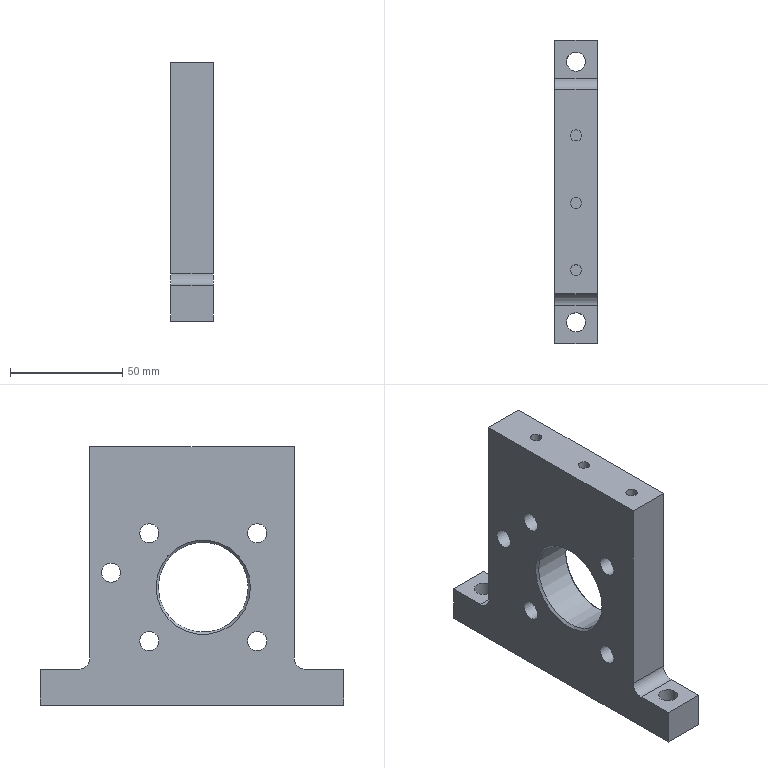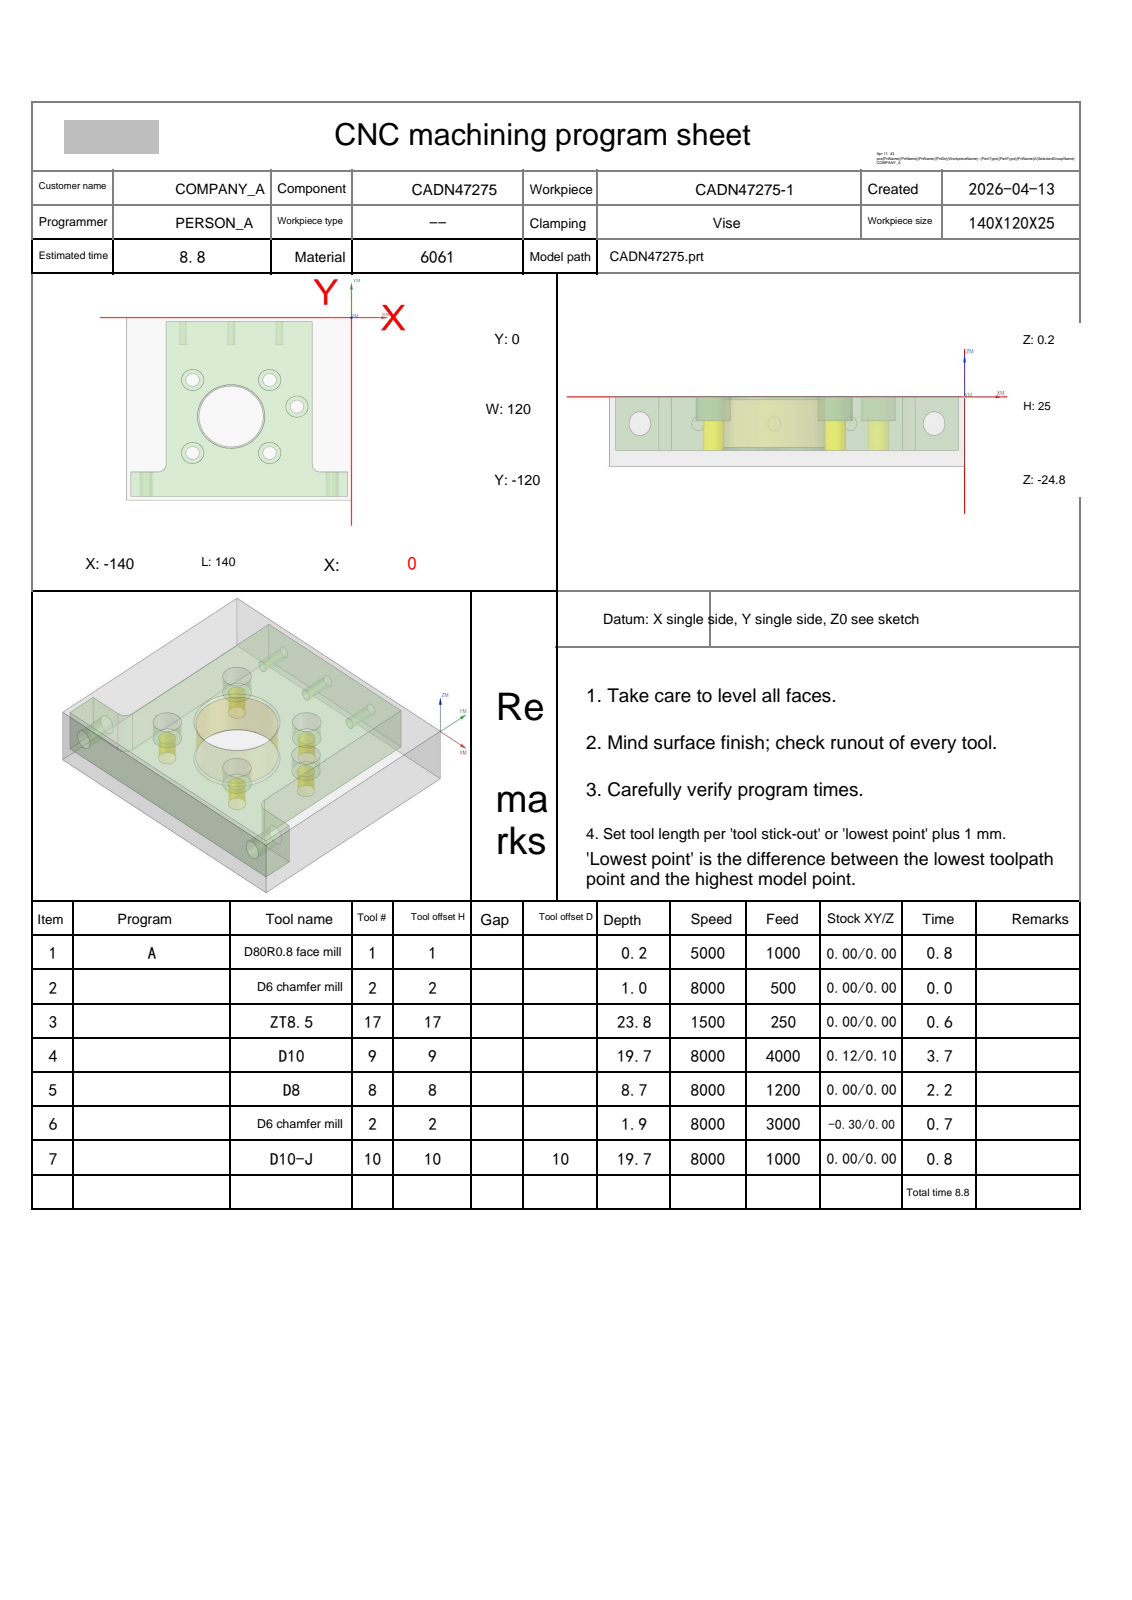NC program | NX | posted by the shop | part box 19 x 135 x 115 mm
Lines 73 to 878 of 2456:
N4 T09 M06
(D10  D=10. R=0. H=09 ce=0.12 di=0.10)
G00 G90 G54 X-117.765 Y10.948 M03 S8000
G43 H09 Z20.
M08
Z-17.5
G01 X-117.749 Y10.849 Z-18.125 F4000.
X-117.733 Y10.75 Z-18.372
X-117.717 Y10.651 Z-18.554
X-117.701 Y10.553 Z-18.7
X-117.686 Y10.454 Z-18.823
X-117.67 Y10.355 Z-18.928
X-117.654 Y10.256 Z-19.02
X-117.638 Y10.158 Z-19.1
X-117.622 Y10.059 Z-19.17
X-117.606 Y9.96 Z-19.232
X-117.591 Y9.861 Z-19.286
X-117.575 Y9.763 Z-19.333
X-117.559 Y9.664 Z-19.374
X-117.543 Y9.565 Z-19.408
X-117.527 Y9.466 Z-19.436
X-117.511 Y9.368 Z-19.46
X-117.496 Y9.269 Z-19.477
X-117.48 Y9.17 Z-19.49
X-117.464 Y9.072 Z-19.497
X-117.448 Y8.973 Z-19.5
X-117.115 Y6.898
G03 X-116.786 Y6.503 I.503 J.083
X-112.933 Y5.928 I3.896 J12.905
X-103.721 Y5.791 I9.212 J309.636
X-101.259 Y5.8 I0.0 J309.773
G01 X-1.649 Y5.779
G02 X4.276 Y1.747 I-.206 J-6.674
X5.587 Y-3.961 I-14.753 J-6.393
X5.818 Y-12.935 I-174.896 J-8.974
X5.799 Y-15.507 I-175.126 J0.0
G01 X5.781 Y-118.297
G02 X1.748 Y-124.273 I-6.683 J.161
X-4.16 Y-125.602 I-6.488 J15.041
X-12.594 Y-125.81 I-8.434 J170.831
X-14.656 Y-125.798 I0.0 J171.039
G01 X-138.297 Y-125.781
G02 X-144.238 Y-121.823 I.146 J6.657
X-145.585 Y-116.06 I14.526 J6.436
X-145.813 Y-107.504 I160.495 J8.556
X-145.798 Y-105.284 I160.723 J0.0
G01 X-145.781 Y-1.693
G02 X-141.823 Y4.238 I6.655 J-.155
X-136.06 Y5.585 I6.436 J-14.523
X-127.504 Y5.813 I8.556 J-160.448
X-125.284 Y5.798 I0.0 J-160.676
X-123.011 Y5.822 I2.274 J-109.436
X-118.506 Y5.729 I0.0 J-109.459
G03 X-106.031 Y5.096 I12.475 J122.585
X-104.399 Y5.107 I0.0 J123.218
G01 X-3.411 Y5.075
G02 X3.002 Y.933 I-.447 J-7.728
X4.757 Y-5.231 I-14.161 J-7.365
X5.1 Y-13.496 I-99.345 J-8.265
X5.092 Y-14.811 I-99.688 J0.0
G01 X5.074 Y-116.58
G02 X.94 Y-122.995 I-7.729 J.44
X-5.348 Y-124.769 I-7.415 J14.255
X-14.012 Y-125.108 I-8.663 J110.618
X-15.769 Y-125.094 I0.0 J110.957
G01 X-136.58 Y-125.075
G02 X-142.999 Y-120.933 I.442 J7.732
X-144.763 Y-114.711 I14.206 J7.389
X-145.108 Y-106.007 I109.485 J8.704
X-145.094 Y-104.22 I109.83 J0.0
G01 X-145.075 Y-3.421
G02 X-140.934 Y2.999 I7.732 J-.442
X-134.711 Y4.763 I7.389 J-14.206
X-126.007 Y5.108 I8.704 J-109.476
X-124.22 Y5.094 I0.0 J-109.822
X-123.6 Y5.096 I.621 J-97.505
X-114.73 Y4.692 I0.0 J-97.507
G03 X-101.233 Y4.378 I13.497 J290.058
X-97.619 Y4.4 I0.0 J290.372
G01 X-5.229 Y4.376
G02 X2.335 Y-.655 I-.393 J-8.793
X4.053 Y-7.188 I-16.636 J-7.866
X4.409 Y-16.533 I-122.28 J-9.345
X4.394 Y-18.449 I-122.636 J0.0
G01 X4.382 Y-114.618
G02 X-.61 Y-122.312 I-8.787 J.235
X-7.415 Y-124.077 I-7.997 J16.841
X-16.317 Y-124.402 I-8.902 J121.564
X-17.836 Y-124.393 I0.0 J121.89
G01 X-134.726 Y-124.377
G02 X-142.28 Y-119.452 I.335 J8.769
X-144.063 Y-112.726 I16.488 J7.97
X-144.403 Y-103.746 I118.292 J8.98
X-144.393 Y-102.165 I118.632 J0.0
G01 X-144.378 Y-5.296
G02 X-139.442 Y2.284 I8.772 J-.316
X-132.847 Y4.049 I7.909 J-16.35
X-124.174 Y4.389 I8.673 J-110.21
X-115.157 Y4.021 I0.0 J-110.55
G03 X-100.288 Y3.681 I14.869 J324.895
X-96.709 Y3.701 I0.0 J325.236
G01 X-7.049 Y3.681
G02 X1.652 Y-2.054 I-.105 J-9.628
X3.357 Y-8.949 I-18.697 J-8.279
X3.703 Y-18.312 I-126.459 J-9.363
X3.692 Y-19.93 I-126.806 J0.0
G01 X3.673 Y-113.09
G02 X2.629 Y-117.342 I-10.374 J.293
G01 X2.446 Y-118.825
X1.934 Y-120.06
X1.12 Y-121.12
X.06 Y-121.934
X-1.175 Y-122.446
G02 X-7.426 Y-123.31 I-30.17 J195.191
X-16.688 Y-123.691 I-9.262 J112.323
X-17.845 Y-123.685 I0.0 J112.704
G01 X-133.055 Y-123.675
G02 X-137.306 Y-122.637 I.246 J10.232
G01 X-138.825 Y-122.446
X-140.06 Y-121.934
X-141.12 Y-121.12
X-141.934 Y-120.06
X-142.446 Y-118.825
G02 X-143.325 Y-112.412 I170.804 J26.702
X-143.69 Y-103.297 I113.665 J9.114
X-143.685 Y-102.201 I114.03 J0.0
G01 X-143.675 Y-6.942
G02 X-138.045 Y1.605 I9.591 J-.19
X-130.95 Y3.366 I8.398 J-18.657
X-123.494 Y3.643 I7.456 J-100.085
X-116.15 Y3.374 I0.0 J-100.362
G03 X-100.164 Y2.992 I15.985 J333.927
X-97.476 Y3.003 I0.0 J334.31
G01 X-8.589 Y2.979
X-8.52
G02 X.904 Y-3.204 I0.0 J-10.273
X2.638 Y-10.315 I-19.87 J-8.614
X3.005 Y-20.222 I-133.631 J-9.907
X2.992 Y-22.066 I-133.997 J0.0
G01 X2.975 Y-111.446
G02 X2.62 Y-114.231 I-16.771 J.721
G01 Y-117.451
X2.6 Y-101.248
G02 X2.418 Y-92.233 I223.082 J9.015
X2.438 Y-89.199 I223.264 J0.0
G01 X2.412 Y-18.929
G03 X2.416 Y-18.177 I-74.932 J.752
X1.871 Y-9.151 I-74.936 J0.0
X-.404 Y-2.515 I-16.313 J-1.884
X-7.619 Y1.981 I-8.589 J-5.744
X-14.302 Y2.433 I-6.683 J-49.236
X-15.228 Y2.424 I0.0 J-49.687
G01 X-23.232 Y2.453
X-24.498 Y2.62
X-111.45 Y2.637
G03 X-122.827 Y3.064 I-32.033 J-701.248
X-124.452 Y3.087 I-1.624 J-58.302
X-132.808 Y2.485 I0.0 J-58.324
X-139. Y.03 I1.969 J-14.001
X-142.642 Y-6.263 I6.083 J-7.72
X-143.124 Y-12.812 I44.253 J-6.549
X-143.117 Y-13.589 I44.735 J0.0
G01 X-143.122 Y-102.549
G03 X-143.124 Y-103.244 I102.156 J-.695
X-142.62 Y-113.38 I102.159 J0.0
X-142.622 Y-114.241 I206.235 J-.861
X-142.593 Y-117.707 I206.237 J0.0
G02 X-142.644 Y-109.06 I731.512 J8.646
X-142.602 Y-101.255 I731.563 J0.0
G03 X-142.42 Y-91.963 I-236.462 J9.292
X-142.439 Y-88.959 I-236.644 J0.0
G01 X-142.411 Y-13.799
G02 X-142.417 Y-13.147 I36.869 J.652
X-141.884 Y-6.9 I36.875 J0.0
X-135.596 Y.566 I10.06 J-2.091
X-128.166 Y2.152 I8.497 J-21.614
X-122.442 Y2.315 I5.724 J-100.129
X-117.463 Y2.192 I0.0 J-100.293
G01 X-116.825 Y2.446
X-115.5 Y2.62
X-110.6
X-115.5
X-116.825 Y2.446
G02 X-119.457 Y1.884 I-2.632 J5.889
G01 X-119.521
G03 X-127.461 Y1.602 I8.321 J-345.796
X-134.633 Y.146 I.995 J-23.303
X-141.052 Y-7.4 I3.89 J-9.811
X-141.812 Y-14.379 I31.689 J-6.979
G01 X-141.811 Y-14.416
G03 X-141.878 Y-23.452 I611.6 J-9.036
G01 Y-23.935
X-141.903 Y-96.2
X-141.986 Y-99.065
X-142.446 Y-100.175
X-142.62 Y-101.498
X-142.446 Y-100.175
G03 X-141.369 Y-95.763 I-9.61 J4.682
X-141.157 Y-86.224 I-214.123 J9.539
X-141.179 Y-83.149 I-214.336 J0.0
G01 X-141.153 Y-17.299
G02 X-141.158 Y-16.586 I47.599 J.713
X-140.605 Y-9.348 I47.605 J0.0
X-133.325 Y-.537 I10.988 J-1.667
X-125.581 Y.915 I8.624 J-24.603
G03 X-119.221 Y1.285 I-3.802 J120.446
X-118.746 Y1.408 I-.724 J3.774
G02 X-117.413 Y2.202 I2.466 J-2.623
G03 X-118.861 Y1.327 I1.415 J-3.975
G02 X-122.098 Y.648 I-3.695 J9.56
G03 X-129.166 Y-.107 I5.054 J-80.754
X-135.663 Y-2.748 I2.192 J-14.706
X-139.753 Y-9.419 I7.358 J-9.102
X-140.551 Y-17. I35.609 J-7.581
G01 Y-17.062
G03 X-140.621 Y-26.574 I650.029 J-9.512
X-140.619 Y-28.262 I650.098 J0.0
G01 X-140.64 Y-89.905
G02 X-140.634 Y-90.696 I-51.361 J-.791
X-141.032 Y-97.077 I-51.367 J0.0
X-141.289 Y-98.099 I-9.752 J1.908
G01 X-141.934 Y-98.94
G03 X-140.422 Y-95.635 I-4.312 J3.971
X-139.944 Y-88.558 I-52.134 J7.077
X-139.949 Y-87.862 I-52.612 J0.0
G01 X-139.919 Y-80.069
X-139.896 Y-20.299
G02 X-139.901 Y-19.504 I57.612 J.795
X-139.372 Y-11.713 I57.618 J0.0
X-136.544 Y-5.179 I12.864 J-1.688
X-129.85 Y-1.255 I9.751 J-8.962
X-122.83 Y-.138 I11.027 J-46.668
G03 X-119.582 Y.565 I-.917 J12.106
G01 X-119.12 Y1.12
X-118.787 Y1.376
G03 X-119.568 Y.549 I1.666 J-2.353
G02 X-122.371 Y-.46 I-3.785 J6.115
G03 X-128.451 Y-1.565 I21.205 J-133.959
X-134.951 Y-4.83 I2.834 J-13.749
X-138.541 Y-11.604 I9.17 J-9.198
X-139.296 Y-19.534 I41.283 J-7.931
G01 Y-19.605
G03 X-139.362 Y-28.974 I663.981 J-9.369
X-139.359 Y-31.085 I664.047 J0.0
G01 X-139.387 Y-87.235
G02 X-139.382 Y-87.963 I-53.015 J-.728
X-139.882 Y-95.231 I-53.02 J0.0
X-140.614 Y-97.486 I-5.927 J.677
G03 X-141.206 Y-97.991 I3.392 J-4.573
G02 X-140.405 Y-97.289 I14.74 J-15.998
G03 X-139.267 Y-94.257 I-5.969 J3.972
X-138.698 Y-86.622 I-50.989 J7.635
X-138.701 Y-86.132 I-51.558 J0.0
G01 X-138.659 Y-76.639
X-138.63 Y-22.199
G02 X-138.634 Y-21.504 I56.935 J.695
X-138.045 Y-13.338 I56.94 J0.0
X-135.069 Y-6.568 I13.543 J-1.916
X-128.639 Y-2.62 I10.123 J-9.278
X-122.69 Y-1.216 I22.71 J-82.942
G03 X-120.094 Y-.232 I-1.362 J7.512
G02 X-119.508 Y.615 I6.338 J-3.753
G03 X-120.062 Y-.228 I2.013 J-1.925
G02 X-122.36 Y-1.48 I-3.707 J4.07
X-127.602 Y-2.946 I-170.119 J597.953
G03 X-133.909 Y-6.609 I3.794 J-13.795
X-137.334 Y-13.709 I10.531 J-9.457
X-138.054 Y-22.224 I49.956 J-8.516
X-138.053 Y-22.627 I50.677 J0.0
G01 X-138.098 Y-33.197
X-138.123 Y-84.303
G02 X-138.118 Y-85.132 I-66.162 J-.829
X-138.631 Y-93.357 I-66.168 J0.0
X-139.784 Y-96.887 I-9.08 J1.014
G01 X-140.615 Y-97.492
G02 X-139.688 Y-96.85 I7.556 J-9.916
G03 X-138.317 Y-94.06 I-4.58 J3.982
X-137.523 Y-87.184 I-32.779 J7.27
X-137.398 Y-77.029 I-413.126 J10.155
X-137.399 Y-76.078 I-413.251 J0.0
G01 X-137.371 Y-24.499
G02 X-137.375 Y-23.813 I63.68 J.686
X-136.81 Y-15.354 I63.684 J0.0
X-133.978 Y-8.337 I14.855 J-1.916
X-127.726 Y-3.994 I10.984 J-9.139
X-122.562 Y-2.227 I219.311 J-632.563
G03 X-120.383 Y-.991 I-1.956 J5.989
G01 X-120.02 Y-.147
G02 X-120.656 Y-1.36 I-3.161 J.885
X-123.65 Y-3.049 I-5.86 J6.888
G03 X-129.001 Y-5.287 I15.603 J-44.831
X-135.744 Y-14.038 I6.275 J-11.808
X-136.739 Y-22.431 I36.853 J-8.623
X-136.841 Y-33.358 I586.61 J-10.927
X-136.838 Y-35.03 I586.712 J0.0
G01 X-136.863 Y-82.133
G02 X-136.859 Y-82.953 I-74.133 J-.82
X-137.394 Y-91.848 I-74.138 J0.0
X-138.784 Y-96.179 I-11.097 J1.171
X-139.284 Y-96.744 I-2.233 J1.473
G01 X-139.93 Y-97.012
G03 X-137.96 Y-95.261 I-.857 J2.948
X-136.595 Y-90.037 I-13.933 J6.431
X-136.142 Y-80.198 I-106.661 J9.839
X-136.15 Y-78.861 I-107.114 J0.0
G01 X-136.111 Y-26.609
G02 X-136.115 Y-25.885 I68.297 J.723
X-135.55 Y-17.114 I68.301 J0.0
X-132.739 Y-9.856 I15.927 J-1.995
X-126.916 Y-5.314 I12.166 J-9.595
G03 X-122.261 Y-3.117 I-40.267 J91.322
X-120.55 Y-1.754 I-2.449 J4.831
G02 X-120.365 Y-.981 I5.741 J-.964
G03 X-120.529 Y-1.76 I2.865 J-1.011
G02 X-122.418 Y-3.567 I-4.172 J2.47
X-127.095 Y-6.075 I-71.012 J126.807
G03 X-134.571 Y-16.003 I6.858 J-12.944
X-135.495 Y-24.829 I42.548 J-8.914
X-135.581 Y-35.581 I671.696 J-10.752
X-135.579 Y-37.358 I671.782 J0.0
G01 X-135.605 Y-80.312
G02 X-135.601 Y-81.068 I-80.89 J-.756
X-136.158 Y-90.54 I-80.893 J0.0
X-137.665 Y-95.46 I-13.433 J1.423
X-138.61 Y-96.515 I-2.353 J1.157
G03 X-139.278 Y-96.742 I1.005 J-4.058
G02 X-138.371 Y-96.435 I5.249 J-14.004
G03 X-136.613 Y-94.133 I-2.8 J3.961
X-135.291 Y-88.226 I-18.857 J7.321
X-134.882 Y-77.993 I-127.868 J10.233
X-134.889 Y-76.694 I-128.276 J0.0
G01 X-134.853 Y-28.699
G02 X-134.858 Y-27.848 I71.97 J.852
X-134.267 Y-18.645 I71.975 J0.0
X-131.423 Y-11.172 I16.89 J-2.151
X-125.809 Y-6.364 I14.236 J-10.94
G03 X-121.657 Y-3.718 I-15.645 J29.138
X-120.62 Y-2.498 I-1.855 J2.628
G01 X-120.51 Y-1.666
G02 X-120.868 Y-3.1 I-3.148 J.023
X-123.427 Y-5.434 I-7.188 J5.311
G03 X-128.253 Y-8.845 I25.166 J-40.716
X-133.408 Y-17.974 I10.642 J-12.03
X-134.25 Y-27.174 I49.857 J-9.201
G01 Y-27.232
G03 X-134.322 Y-37.062 I675.106 J-9.83
X-134.318 Y-39.201 I675.177 J0.0
G01 X-134.342 Y-78.217
G02 X-134.338 Y-79.102 I-91.498 J-.885
X-134.901 Y-89.242 I-91.502 J0.0
X-136.475 Y-94.724 I-16.019 J1.63
X-137.96 Y-96.423 I-3.994 J1.994
G01 X-138.608 Y-96.526
G03 X-136.597 Y-95.433 I-.071 J2.526
X-134.637 Y-90.879 I-8.843 J6.505
X-133.725 Y-81.624 I-49.778 J9.582
X-133.616 Y-69.483 I-680.04 J12.141
X-133.619 Y-67.679 I-680.148 J0.0
G01 X-133.593 Y-30.599
G02 X-133.598 Y-29.747 I77.428 J.852
X-133.024 Y-20.333 I77.433 J0.0
X-130.071 Y-12.33 I18.219 J-2.176
X-125.24 Y-7.643 I16.579 J-12.255
G03 X-121.461 Y-4.592 I-15.484 J23.044
X-120.62 Y-3.311 I-2.183 J2.35
G01 Y-2.498
G02 X-120.597 Y-2.878 I-3.103 J-.379
X-120.74 Y-3.813 I-3.126 J0.0
X-122.888 Y-6.38 I-6.976 J3.656
G03 X-127.248 Y-10.112 I49.65 J-62.404
X-132.236 Y-19.88 I12.635 J-12.609
X-133.008 Y-29.46 I59.051 J-9.58
G01 X-133.007 Y-29.778
X-133.058 Y-40.348
X-133.09 Y-77.368
G02 X-133.088 Y-78.015 I-88.984 J-.646
X-133.71 Y-88.516 I-88.986 J0.0
X-135.406 Y-94.303 I-17.215 J1.904
X-137.277 Y-96.356 I-4.353 J2.09
G01 X-137.984 Y-96.444
G03 X-136.757 Y-96.183 I-.026 J3.141
X-134.502 Y-93.4 I-3.352 J5.022
X-132.906 Y-86.959 I-19.948 J8.361
X-132.369 Y-75.752 I-116.747 J11.208
X-132.376 Y-74.515 I-117.284 J0.0
G01 X-132.335 Y-32.559
G02 X-132.341 Y-31.616 I83.331 J.943
X-131.769 Y-21.872 I83.337 J0.0
X-128.527 Y-13.084 I19.623 J-2.248
X-124.543 Y-8.801 I20.693 J-15.254
G03 X-121.247 Y-5.515 I-15.725 J19.071
X-120.62 Y-4.392 I-2.744 J2.268
G01 Y-3.342
G02 X-120.595 Y-3.82 I-4.597 J-.478
X-120.721 Y-4.892 I-4.622 J0.0
X-122.848 Y-7.823 I-8.328 J3.804
G03 X-127.032 Y-12.235 I38.892 J-41.084
X-131.081 Y-21.879 I16.035 J-12.404
X-131.763 Y-31.776 I71.49 J-9.896
X-131.761 Y-32.348 I72.171 J0.0
G01 X-131.798 Y-41.728
X-131.83 Y-75.83
G02 X-131.828 Y-76.434 I-97.356 J-.604
X-132.443 Y-87.358 I-97.358 J0.0
X-134.217 Y-93.738 I-19.736 J2.051
X-136.536 Y-96.328 I-5.282 J2.396
X-137.116 Y-96.391 I-.58 J2.631
X-137.364 Y-96.38 I0.0 J2.694
G03 X-137.071 Y-96.396 I.293 J2.689
X-134.989 Y-95.418 I0.0 J2.705
X-132.623 Y-90.975 I-7.865 J7.04
X-131.342 Y-82.207 I-37.962 J10.022
X-131.078 Y-68.57 I-351.279 J13.637
X-131.099 Y-64.739 I-351.543 J0.0
G01 X-131.067 Y-33.389
G02 X-131.07 Y-32.708 I77.963 J.681
X-130.443 Y-22.846 I77.966 J0.0
X-124.736 Y-10.903 I21.006 J-2.704
G03 X-121.445 Y-7.153 I-36.854 J35.658
X-120.62 Y-5.66 I-4.069 J3.224
G01 Y-4.4
G02 X-120.606 Y-4.926 I-10.368 J-.526
X-120.662 Y-5.997 I-10.381 J0.0
X-122.432 Y-8.994 I-8.28 J2.868
G03 X-126.296 Y-13.854 I50.804 J-44.367
X-129.897 Y-23.705 I19.228 J-12.61
X-130.511 Y-33.897 I84.208 J-10.191
X-130.508 Y-34.6 I84.823 J0.0
G01 X-130.57 Y-74.43
G02 X-130.569 Y-75.016 I-103.991 J-.586
X-131.193 Y-86.394 I-103.993 J0.0
X-133.028 Y-93.232 I-22.037 J2.247
X-135.59 Y-96.24 I-6.198 J2.684
X-136.367 Y-96.403 I-.778 J1.764
X-136.667 Y-96.38 I0.0 J1.928
G03 X-136.302 Y-96.403 I.365 J2.858
X-134.17 Y-95.46 I0.0 J2.881
X-131.587 Y-90.934 I-7.673 J7.38
X-130.164 Y-82.358 I-35.447 J10.287
X-129.826 Y-69.46 I-246.174 J12.898
X-129.84 Y-66.836 I-246.511 J0.0
G01 X-129.807 Y-35.079
G02 X-129.811 Y-34.292 I81.22 J.787
X-129.154 Y-23.977 I81.223 J0.0
X-123.874 Y-11.984 I23.956 J-3.387
G03 X-120.94 Y-7.879 I-24.384 J20.527
X-120.62 Y-7.125 I-6.574 J3.24
G01 Y-5.725
G02 X-120.595 Y-6.353 I-8.078 J-.627
X-120.7 Y-7.652 I-8.102 J0.0
X-122.543 Y-11.002 I-11.461 J4.123
G03 X-126.28 Y-16.899 I33.565 J-25.402
X-128.869 Y-26.947 I26.069 J-12.075
X-129.279 Y-37.818 I144.056 J-10.872
X-129.269 Y-39.466 I144.465 J0.0
G01 X-129.312 Y-73.239
G02 X-129.31 Y-73.885 I-105.368 J-.647
X-129.995 Y-85.883 I-105.37 J0.0
X-131.925 Y-92.952 I-23.144 J2.52
X-134.582 Y-96.149 I-6.926 J3.054
X-135.127 Y-96.38 I-2.219 J4.473
G01 X-135.897
G03 X-135.511 Y-96.404 I.386 J3.15
X-133.129 Y-95.326 I0.0 J3.173
X-130.454 Y-90.631 I-8.315 J7.847
X-128.924 Y-81.582 I-36.736 J10.864
X-128.566 Y-68.277 I-247.222 J13.305
X-128.58 Y-65.646 I-247.58 J0.0
G01 X-128.548 Y-36.689
G02 X-128.552 Y-35.921 I87.819 J.768
X-127.916 Y-25.375 I87.822 J0.0
X-123.298 Y-13.454 I27.16 J-3.667
G03 X-120.766 Y-9.237 I-26.882 J19.005
G01 X-120.62 Y-8.815
Y-7.135
G02 X-120.596 Y-7.878 I-11.841 J-.743
X-120.688 Y-9.346 I-11.864 J0.0
X-122.359 Y-12.871 I-13.667 J4.322
G03 X-125.961 Y-20.079 I32.279 J-20.636
X-127.775 Y-30.387 I36.188 J-11.682
X-128.036 Y-42.916 I300.505 J-12.529
X-128.018 Y-46.273 I300.766 J0.0
G01 X-128.051 Y-71.91
G02 X-128.049 Y-72.534 I-113.352 J-.623
X-128.729 Y-84.926 I-113.354 J0.0
X-130.693 Y-92.451 I-25.69 J2.686
X-133.512 Y-96.039 I-7.935 J3.334
X-134.236 Y-96.38 I-1.806 J2.895
G01 X-135.006
G03 X-134.618 Y-96.403 I.388 J3.223
X-132.236 Y-95.363 I0.0 J3.246
X-129.404 Y-90.616 I-8.262 J8.146
X-127.758 Y-81.801 I-35.035 J11.104
X-127.319 Y-68.782 I-192.735 J13.019
X-127.326 Y-67.108 I-193.174 J0.0
G01 X-127.284 Y-37.809
G02 X-127.287 Y-37.153 I88.854 J.656
X-126.629 Y-26.356 I88.857 J0.0
X-122.658 Y-14.91 I31.2 J-4.411
G03 X-120.629 Y-10.828 I-25.961 J15.45
G01 X-120.62 Y-8.878
G02 X-120.602 Y-9.691 I-18.653 J-.813
X-120.671 Y-11.29 I-18.671 J0.0
X-122.079 Y-14.841 I-15.855 J4.233
G03 X-125.486 Y-23.766 I34.398 J-18.244
X-126.651 Y-34.817 I55.984 J-11.489
X-126.763 Y-47.611 I729.032 J-12.795
X-126.758 Y-50.286 I729.144 J0.0
G01 X-126.789 Y-70.513
G02 X-126.787 Y-71.229 I-120.917 J-.716
X-127.474 Y-84.1 I-120.919 J0.0
X-129.5 Y-92.064 I-27.833 J2.839
X-132.48 Y-95.969 I-8.672 J3.53
X-133.324 Y-96.38 I-1.916 J2.858
G01 X-134.164
G03 X-133.745 Y-96.404 I.418 J3.602
X-132.498 Y-96.183 I0.0 J3.626
X-129.633 Y-93.324 I-3.37 J6.243
X-127.211 Y-86.36 I-18.481 J10.329
X-126.168 Y-74.291 I-76.073 J12.654
X-126.054 Y-61.379 I-728.545 J12.912
X-126.058 Y-58.789 I-728.66 J0.0
G01 X-126.019 Y-38.719
G02 X-126.021 Y-38.15 I86.559 J.569
X-125.28 Y-26.852 I86.561 J0.0
X-122.083 Y-16.595 I36.34 J-5.7
G03 X-120.62 Y-13.061 I-30.068 J14.52
G01 Y-10.891
G02 X-120.598 Y-11.901 I-23.36 J-1.011
X-120.663 Y-13.649 I-23.382 J0.0
X-121.851 Y-17.278 I-20.317 J4.64
G03 X-125.252 Y-32.783 I40.913 J-17.1
X-125.518 Y-46.361 I346.221 J-13.578
X-125.498 Y-50.139 I346.488 J0.0
G01 X-125.537 Y-70.017
X-125.536 Y-70.483
G02 X-126.256 Y-83.601 I-119.758 J0.0
X-128.426 Y-91.969 I-28.723 J2.982
X-131.529 Y-95.972 I-8.927 J3.716
X-132.376 Y-96.38 I-2.015 J3.098
G01 X-133.216
G03 X-132.796 Y-96.405 I.42 J3.535
X-131.416 Y-96.127 I0.0 J3.56
X-128.459 Y-93.063 I-3.854 J6.678
X-125.97 Y-85.75 I-19.93 J10.864
X-124.923 Y-73.792 I-77.898 J12.85
X-124.774 Y-56.93 I-958.052 J16.861
X-124.798 Y-50.259 I-958.2 J0.0
G02 X-124.818 Y-46.608 I333.628 J3.651
X-124.547 Y-33.183 I333.648 J0.0
X-121.369 Y-18.061 I46.479 J-1.875
G01 X-120.62 Y-15.829
Y-13.239
G02 X-120.599 Y-14.409 I-33.203 J-1.171
X-120.676 Y-16.668 I-33.224 J0.0
X-122.064 Y-21.803 I-49.652 J10.669
G03 X-124.053 Y-35.131 I52.99 J-14.721
X-124.248 Y-48.026 I426.064 J-12.895
X-124.237 Y-51.089 I426.259 J0.0
G02 X-124.216 Y-57.133 I-858.545 J-6.044
X-124.387 Y-74.266 I-858.566 J0.0
X-125.583 Y-86.383 I-72.445 J1.034
X-128.198 Y-93.435 I-21.021 J3.783
X-131.186 Y-96.317 I-6.44 J3.687
X-131.908 Y-96.398 I-.722 J3.192
X-132.246 Y-96.38 I0.0 J3.273
G03 X-131.824 Y-96.405 I.422 J3.565
X-130.43 Y-96.123 I0.0 J3.59
X-127.348 Y-92.928 I-3.988 J6.931
X-124.788 Y-85.484 I-20.625 J11.254
X-123.667 Y-72.95 I-79.163 J13.398
X-123.526 Y-57.632 I-829.623 J15.318
X-123.538 Y-53.059 I-829.765 J0.0
G02 X-123.557 Y-49.024 I424.71 J4.035
X-123.326 Y-35.012 I424.729 J0.0
X-120.756 Y-19.878 I60.069 J-2.418
G01 X-120.62 Y-19.332
Y-16.042
G02 X-120.598 Y-17.665 I-59.766 J-1.623
X-120.662 Y-20.435 I-59.788 J0.0
X-121.757 Y-26.275 I-126.534 J20.71
G03 X-122.908 Y-40.072 I83.63 J-13.921
X-123.002 Y-53.648 I980.153 J-13.577
X-122.98 Y-60.195 I980.248 J0.0
G02 X-122.965 Y-63.125 I-284.236 J-2.931
X-123.353 Y-77.97 I-284.251 J0.0
X-125.049 Y-88.657 I-49.408 J2.363
X-128.082 Y-94.654 I-15.786 J4.218
X-130.413 Y-96.38 I-4.217 J3.258
G01 X-131.323
G03 X-130.875 Y-96.405 I.448 J4.059
X-129.614 Y-96.205 I0.0 J4.084
X-126.588 Y-93.378 I-3.322 J6.589
X-123.782 Y-86.091 I-18.67 J11.374
X-122.475 Y-74.023 I-69.198 J13.596
X-122.255 Y-57.204 I-642.881 J16.819
X-122.277 Y-51.939 I-643.101 J0.0
G02 X-122.294 Y-48.601 I325.981 J3.338
X-122.01 Y-35.003 I325.998 J0.0
X-120.62 Y-24.227 I73.569 J-4.015
G01 Y-19.887
G02 X-120.599 Y-22.202 I-127.207 J-2.315
X-120.673 Y-26.562 I-127.228 J0.0
G03 X-121.712 Y-45.035 I163.785 J-18.472
X-121.704 Y-46.666 I164.823 J0.0
G01 X-121.764 Y-67.423
X-121.763 Y-67.67
G02 X-122.533 Y-81.791 I-129.944 J0.0
X-124.842 Y-91.055 I-33.79 J3.502
X-128.109 Y-95.659 I-11.084 J4.405
X-129.413 Y-96.38 I-2.661 J3.273
G01 X-130.323
G03 X-129.881 Y-96.401 I.442 J4.599
X-128.742 Y-96.259 I0.0 J4.621
X-125.816 Y-93.772 I-2.784 J6.242
X-122.853 Y-86.916 I-16.71 J11.291
X-121.316 Y-75.136 I-59.095 J13.696
X-121. Y-59.449 I-388.903 J15.687
X-121.019 Y-55.636 I-389.219 J0.0
G02 X-121.037 Y-51.599 I450.973 J4.037
X-120.785 Y-36.539 I450.991 J0.0
G01 X-120.62 Y-33.795
Y-25.535
X-120.638 Y-71.775
G02 X-121.864 Y-84.812 I-81.446 J1.082
X-124.637 Y-92.745 I-25.053 J4.306
X-127.791 Y-96.13 I-8.056 J4.343
X-128.391 Y-96.38 I-3.504 J7.577
G01 X-129.301
G03 X-128.852 Y-96.404 I.448 J4.155
X-127.572 Y-96.203 I0.0 J4.18
X-124.444 Y-93.322 I-3.414 J6.844
X-121.46 Y-85.829 I-19.211 J11.991
X-120.62 Y-81.031 I-62.368 J13.388
G01 Y-70.951
G02 X-120.601 Y-75.705 I-586.701 J-4.754
X-120.651 Y-83.416 I-586.72 J0.0
X-123.898 Y-93.264 I-22.423 J1.933
X-127.117 Y-96.308 I-6.959 J4.135
X-127.892 Y-96.402 I-.775 J3.177
X-128.267 Y-96.38 I0.0 J3.27
G03 X-127.819 Y-96.404 I.448 J4.169
X-126.524 Y-96.199 I0.0 J4.193
X-123.37 Y-93.31 I-3.445 J6.928
X-120.62 Y-86.732 I-17.068 J10.999
G01 Y-82.812
G02 X-120.596 Y-84.636 I-68.057 J-1.824
X-120.668 Y-87.769 I-68.081 J0.0
X-124.564 Y-95.304 I-13.315 J2.11
X-126.316 Y-96.38 I-3.352 J3.493
G01 X-127.226
G03 X-126.775 Y-96.404 I.451 J4.179
X-125.474 Y-96.198 I0.0 J4.203
X-122.298 Y-93.276 I-3.425 J6.912
X-120.62 Y-89.744 I-11.587 J7.667
G01 Y-87.154
G02 X-120.602 Y-88.274 I-34.368 J-1.12
X-120.664 Y-90.337 I-34.387 J0.0
X-124.612 Y-96.097 I-8.86 J1.84
X-125.274 Y-96.38 I-3.193 J6.569
G01 X-126.184
G03 X-125.732 Y-96.405 I.452 J4.149
X-124.432 Y-96.197 I0.0 J4.173
X-121.119 Y-92.88 I-3.263 J6.571
X-120.62 Y-91.727 I-9.507 J4.804
G01 Y-89.907
X-120.646 Y-92.063
G02 X-124.216 Y-96.373 I-6.045 J1.374
G01 X-125.171 Y-96.38
G03 X-124.723 Y-96.405 I.448 J4.069
X-123.458 Y-96.204 I0.0 J4.093
X-120.62 Y-93.127 I-2.277 J4.947
G01 Y-91.867
G02 X-120.609 Y-92.369 I-11.694 J-.502
X-120.66 Y-93.461 I-11.705 J0.0
X-123.34 Y-96.38 I-4.188 J1.155
G01 X-124.18
G03 X-123.762 Y-96.405 I.418 J3.484
X-122.528 Y-96.181 I0.0 J3.509
X-120.62 Y-94.131 I-1.484 J3.294
G01 Y-93.151
G02 X-120.596 Y-93.619 I-4.514 J-.468
X-120.676 Y-94.47 I-4.538 J0.0
X-122.568 Y-96.38 I-2.89 J.971
G01 X-123.268
G03 X-122.912 Y-96.404 I.356 J2.672
X-121.781 Y-96.155 I0.0 J2.696
X-120.62 Y-94.843 I-.993 J2.049
G01 Y-94.143
G02 X-120.595 Y-94.478 I-2.237 J-.334
X-120.773 Y-95.358 I-2.261 J0.0
X-121.985 Y-96.38 I-1.782 J.883
G01 X-122.475
G03 X-122.204 Y-96.401 I.271 J1.699
X-120.631 Y-95.378 I0.0 J1.721
G01 X-120.62 Y-94.884
G02 X-120.598 Y-95.122 I-1.278 J-.238
X-121.57 Y-96.38 I-1.3 J0.0
G01 X-121.92
G03 X-121.685 Y-96.405 I.235 J1.096
X-120.62 Y-95.634 I0.0 J1.12
G01 Y-95.354
X-120.603 Y-95.524
G02 X-121.46 Y-96.381 I-.857 J0.0
G01 X-121.502 Y-96.38
X-121.363 Y-96.393
G03 X-120.694 Y-96.007 I0.0 J.774
X-120.633 Y-95.755 I-.489 J.252
X-121.183 Y-95.205 I-.55 J0.0
X-121.541 Y-95.338 I0.0 J-.55
X-121.811 Y-95.819 I.294 J-.481
X-121.427 Y-96.353 I.564 J0.0
G01 X-121.244 Y-96.38
G03 X-120.61 Y-95.746 I0.0 J.634
G01 X-120.62 Y-95.632
G03 X-120.891 Y-95.188 I-.504 J-.003
G01 X-121.611 Y-94.817
X-123.368 Y-93.914 Z-19.4
X-124.24 Y-93.465
X-124.313 Y-93.435
X-124.39 Y-93.416
X-124.469 Y-93.41
X-140.518
X-140.73 Y-93.418
X-140.942 Y-93.44
X-141.151 Y-93.478
X-141.357 Y-93.531
X-141.559 Y-93.598
X-141.756 Y-93.679
X-141.946 Y-93.775
X-142.129 Y-93.883
X-142.304 Y-94.005
X-142.47 Y-94.138
X-142.625 Y-94.283
X-142.868 Y-94.536
X-143.101 Y-94.798
X-143.324 Y-95.068
X-143.536 Y-95.347
X-143.737 Y-95.635
X-143.927 Y-95.929
X-144.105 Y-96.231
X-144.3 Y-96.592
X-144.484 Y-96.959
X-144.656 Y-97.331
X-144.816 Y-97.709
X-144.964 Y-98.091
X-145.099 Y-98.479
X-145.203 Y-98.814
X-145.294 Y-99.152
X-145.373 Y-99.494
X-145.439 Y-99.838
X-145.491 Y-100.185
X-145.531 Y-100.534
X-145.558 Y-100.883
X-146.323 Y-114.175
X-146.341 Y-114.625
X-146.346 Y-115.075
X-146.336 Y-115.526
X-146.312 Y-115.975
X-146.274 Y-116.424
X-146.222 Y-116.871
X-146.155 Y-117.317
X-146.075 Y-117.76
X-145.98 Y-118.2
X-145.872 Y-118.637
X-145.75 Y-119.071
X-145.614 Y-119.5
X-145.387 Y-120.18
X-145.285 Y-120.464
X-145.171 Y-120.743
X-145.044 Y-121.017
X-144.905 Y-121.285
X-144.754 Y-121.546
X-144.592 Y-121.8
X-144.418 Y-122.046
X-144.234 Y-122.285
X-144.038 Y-122.515
X-143.833 Y-122.736
X-143.618 Y-122.948
X-143.394 Y-123.149
X-143.161 Y-123.341
X-141.249 Y-124.842
X-141.182 Y-124.886
X-141.109 Y-124.92
X-141.031 Y-124.941
X-140.95 Y-124.949
X-140.87 Y-124.944
X-140.791 Y-124.926
X-140.716 Y-124.896
X-140.647 Y-124.854
X-140.239 Y-124.558
X-138.639 Y-123.4 Z-19.5
X-137.627 Y-122.674
G02 X-137.229 Y-122.627 I.398 J-1.66
X-136.861 Y-122.667 I0.0 J-1.707
G03 X-129.142 Y-123.139 I7.719 J62.841
X-127.889 Y-123.127 I0.0 J63.313
G01 X-17.019 Y-123.115
G03 X-16.485 Y-123.116 I.534 J98.103
X-6.629 Y-122.62 I0.0 J98.104
G01 X-2.363 Y-122.602
X-2.502 Y-122.62
X-137.389
G03 X-137.805 Y-122.839 I.004 J-.512
G01 X-138.745 Y-124.206
G03 X-138.834 Y-124.492 I.416 J-.286